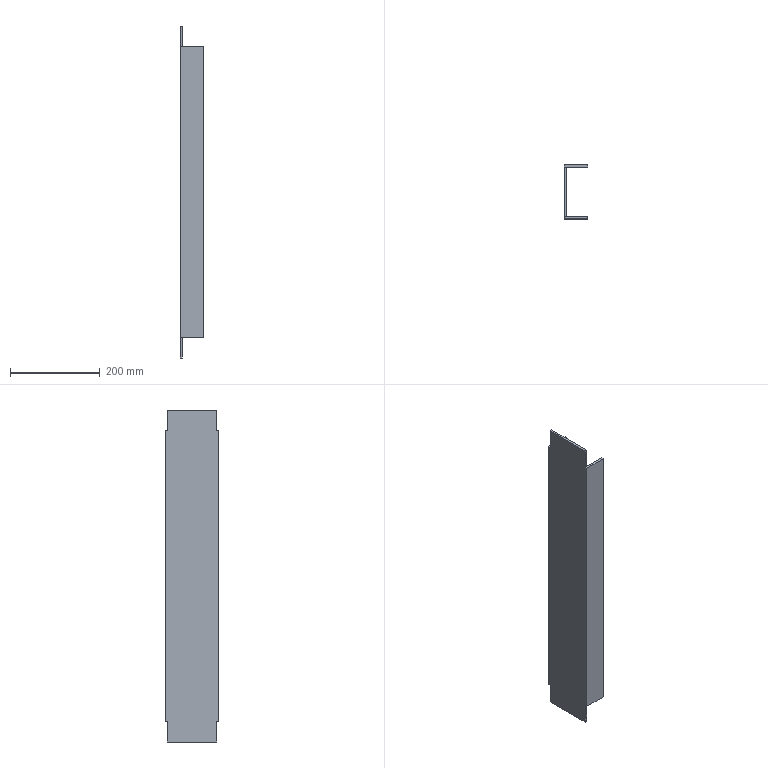Part | SolidWorks | features ICE 3, Extrusion 1 | 1 solid | 18 faces | box 53 x 120 x 740 mm | volume 751500 mm3 | plane 18
STEP:
#1=CARTESIAN_POINT('',(0.,-120.,695.));
#2=VERTEX_POINT('',#1);
#3=CARTESIAN_POINT('',(53.,-120.,695.));
#4=VERTEX_POINT('',#3);
#5=CARTESIAN_POINT('',(53.,-120.,695.));
#6=DIRECTION('',(1.,0.,0.));
#7=VECTOR('',#6,1000.);
#8=LINE('',#5,#7);
#9=EDGE_CURVE('',#2,#4,#8,.T.);
#10=ORIENTED_EDGE('',*,*,#9,.F.);
#11=CARTESIAN_POINT('',(0.,-120.,45.));
#12=VERTEX_POINT('',#11);
#13=CARTESIAN_POINT('',(0.,-120.,740.));
#14=DIRECTION('',(0.,0.,-1.));
#15=VECTOR('',#14,1000.);
#16=LINE('',#13,#15);
#17=EDGE_CURVE('',#2,#12,#16,.T.);
#18=ORIENTED_EDGE('',*,*,#17,.T.);
#19=CARTESIAN_POINT('',(53.,-120.,45.));
#20=VERTEX_POINT('',#19);
#21=CARTESIAN_POINT('',(0.,-120.,45.));
#22=DIRECTION('',(-1.,0.,0.));
#23=VECTOR('',#22,1000.);
#24=LINE('',#21,#23);
#25=EDGE_CURVE('',#20,#12,#24,.T.);
#26=ORIENTED_EDGE('',*,*,#25,.F.);
#27=CARTESIAN_POINT('',(53.,-120.,740.));
#28=DIRECTION('',(0.,0.,-1.));
#29=VECTOR('',#28,1000.);
#30=LINE('',#27,#29);
#31=EDGE_CURVE('',#4,#20,#30,.T.);
#32=ORIENTED_EDGE('',*,*,#31,.F.);
#33=EDGE_LOOP('',(#10,#18,#26,#32));
#34=FACE_OUTER_BOUND('',#33,.T.);
#35=CARTESIAN_POINT('',(0.,-120.,740.));
#36=DIRECTION('',(0.,1.,0.));
#37=DIRECTION('',(0.,0.,1.));
#38=AXIS2_PLACEMENT_3D('',#35,#36,#37);
#39=PLANE('',#38);
#40=ADVANCED_FACE('',(#34),#39,.F.);
#41=CARTESIAN_POINT('',(53.,-115.,695.));
#42=VERTEX_POINT('',#41);
#43=CARTESIAN_POINT('',(53.,-120.,695.));
#44=DIRECTION('',(0.,1.,0.));
#45=VECTOR('',#44,1000.);
#46=LINE('',#43,#45);
#47=EDGE_CURVE('',#4,#42,#46,.T.);
#48=ORIENTED_EDGE('',*,*,#47,.F.);
#49=ORIENTED_EDGE('',*,*,#31,.T.);
#50=CARTESIAN_POINT('',(53.,-115.,45.));
#51=VERTEX_POINT('',#50);
#52=CARTESIAN_POINT('',(53.,-120.,45.));
#53=DIRECTION('',(0.,-1.,0.));
#54=VECTOR('',#53,1000.);
#55=LINE('',#52,#54);
#56=EDGE_CURVE('',#51,#20,#55,.T.);
#57=ORIENTED_EDGE('',*,*,#56,.F.);
#58=CARTESIAN_POINT('',(53.,-115.,740.));
#59=DIRECTION('',(0.,0.,-1.));
#60=VECTOR('',#59,1000.);
#61=LINE('',#58,#60);
#62=EDGE_CURVE('',#42,#51,#61,.T.);
#63=ORIENTED_EDGE('',*,*,#62,.F.);
#64=EDGE_LOOP('',(#48,#49,#57,#63));
#65=FACE_OUTER_BOUND('',#64,.T.);
#66=CARTESIAN_POINT('',(53.,-120.,740.));
#67=DIRECTION('',(-1.,0.,0.));
#68=DIRECTION('',(0.,0.,1.));
#69=AXIS2_PLACEMENT_3D('',#66,#67,#68);
#70=PLANE('',#69);
#71=ADVANCED_FACE('',(#65),#70,.F.);
#72=CARTESIAN_POINT('',(5.,-115.,695.));
#73=VERTEX_POINT('',#72);
#74=CARTESIAN_POINT('',(53.,-115.,695.));
#75=DIRECTION('',(-1.,0.,0.));
#76=VECTOR('',#75,1000.);
#77=LINE('',#74,#76);
#78=EDGE_CURVE('',#42,#73,#77,.T.);
#79=ORIENTED_EDGE('',*,*,#78,.F.);
#80=ORIENTED_EDGE('',*,*,#62,.T.);
#81=CARTESIAN_POINT('',(5.,-115.,45.));
#82=VERTEX_POINT('',#81);
#83=CARTESIAN_POINT('',(53.,-115.,45.));
#84=DIRECTION('',(1.,0.,0.));
#85=VECTOR('',#84,1000.);
#86=LINE('',#83,#85);
#87=EDGE_CURVE('',#82,#51,#86,.T.);
#88=ORIENTED_EDGE('',*,*,#87,.F.);
#89=CARTESIAN_POINT('',(5.,-115.,740.));
#90=DIRECTION('',(0.,0.,-1.));
#91=VECTOR('',#90,1000.);
#92=LINE('',#89,#91);
#93=EDGE_CURVE('',#73,#82,#92,.T.);
#94=ORIENTED_EDGE('',*,*,#93,.F.);
#95=EDGE_LOOP('',(#79,#80,#88,#94));
#96=FACE_OUTER_BOUND('',#95,.T.);
#97=CARTESIAN_POINT('',(5.,-115.,740.));
#98=DIRECTION('',(0.,-1.,0.));
#99=DIRECTION('',(0.,0.,-1.));
#100=AXIS2_PLACEMENT_3D('',#97,#98,#99);
#101=PLANE('',#100);
#102=ADVANCED_FACE('',(#96),#101,.F.);
#103=CARTESIAN_POINT('',(53.,0.,695.));
#104=VERTEX_POINT('',#103);
#105=CARTESIAN_POINT('',(0.,0.,695.));
#106=VERTEX_POINT('',#105);
#107=CARTESIAN_POINT('',(53.,0.,695.));
#108=DIRECTION('',(-1.,0.,0.));
#109=VECTOR('',#108,1000.);
#110=LINE('',#107,#109);
#111=EDGE_CURVE('',#104,#106,#110,.T.);
#112=ORIENTED_EDGE('',*,*,#111,.F.);
#113=CARTESIAN_POINT('',(53.,0.,45.));
#114=VERTEX_POINT('',#113);
#115=CARTESIAN_POINT('',(53.,0.,740.));
#116=DIRECTION('',(0.,0.,-1.));
#117=VECTOR('',#116,1000.);
#118=LINE('',#115,#117);
#119=EDGE_CURVE('',#104,#114,#118,.T.);
#120=ORIENTED_EDGE('',*,*,#119,.T.);
#121=CARTESIAN_POINT('',(0.,0.,45.));
#122=VERTEX_POINT('',#121);
#123=CARTESIAN_POINT('',(53.,0.,45.));
#124=DIRECTION('',(1.,0.,0.));
#125=VECTOR('',#124,1000.);
#126=LINE('',#123,#125);
#127=EDGE_CURVE('',#122,#114,#126,.T.);
#128=ORIENTED_EDGE('',*,*,#127,.F.);
#129=CARTESIAN_POINT('',(0.,0.,740.));
#130=DIRECTION('',(0.,0.,-1.));
#131=VECTOR('',#130,1000.);
#132=LINE('',#129,#131);
#133=EDGE_CURVE('',#106,#122,#132,.T.);
#134=ORIENTED_EDGE('',*,*,#133,.F.);
#135=EDGE_LOOP('',(#112,#120,#128,#134));
#136=FACE_OUTER_BOUND('',#135,.T.);
#137=CARTESIAN_POINT('',(0.,0.,740.));
#138=DIRECTION('',(0.,-1.,0.));
#139=DIRECTION('',(0.,0.,-1.));
#140=AXIS2_PLACEMENT_3D('',#137,#138,#139);
#141=PLANE('',#140);
#142=ADVANCED_FACE('',(#136),#141,.F.);
#143=CARTESIAN_POINT('',(5.,-5.,695.));
#144=VERTEX_POINT('',#143);
#145=CARTESIAN_POINT('',(53.,-5.,695.));
#146=VERTEX_POINT('',#145);
#147=CARTESIAN_POINT('',(0.,-5.,695.));
#148=DIRECTION('',(1.,0.,0.));
#149=VECTOR('',#148,1000.);
#150=LINE('',#147,#149);
#151=EDGE_CURVE('',#144,#146,#150,.T.);
#152=ORIENTED_EDGE('',*,*,#151,.F.);
#153=CARTESIAN_POINT('',(5.,-5.,45.));
#154=VERTEX_POINT('',#153);
#155=CARTESIAN_POINT('',(5.,-5.,740.));
#156=DIRECTION('',(0.,0.,-1.));
#157=VECTOR('',#156,1000.);
#158=LINE('',#155,#157);
#159=EDGE_CURVE('',#144,#154,#158,.T.);
#160=ORIENTED_EDGE('',*,*,#159,.T.);
#161=CARTESIAN_POINT('',(53.,-5.,45.));
#162=VERTEX_POINT('',#161);
#163=CARTESIAN_POINT('',(0.,-5.,45.));
#164=DIRECTION('',(-1.,0.,0.));
#165=VECTOR('',#164,1000.);
#166=LINE('',#163,#165);
#167=EDGE_CURVE('',#162,#154,#166,.T.);
#168=ORIENTED_EDGE('',*,*,#167,.F.);
#169=CARTESIAN_POINT('',(53.,-5.,740.));
#170=DIRECTION('',(0.,0.,-1.));
#171=VECTOR('',#170,1000.);
#172=LINE('',#169,#171);
#173=EDGE_CURVE('',#146,#162,#172,.T.);
#174=ORIENTED_EDGE('',*,*,#173,.F.);
#175=EDGE_LOOP('',(#152,#160,#168,#174));
#176=FACE_OUTER_BOUND('',#175,.T.);
#177=CARTESIAN_POINT('',(5.,-5.,740.));
#178=DIRECTION('',(0.,1.,0.));
#179=DIRECTION('',(0.,0.,1.));
#180=AXIS2_PLACEMENT_3D('',#177,#178,#179);
#181=PLANE('',#180);
#182=ADVANCED_FACE('',(#176),#181,.F.);
#183=CARTESIAN_POINT('',(53.,-5.,695.));
#184=DIRECTION('',(0.,1.,0.));
#185=VECTOR('',#184,1000.);
#186=LINE('',#183,#185);
#187=EDGE_CURVE('',#146,#104,#186,.T.);
#188=ORIENTED_EDGE('',*,*,#187,.F.);
#189=ORIENTED_EDGE('',*,*,#173,.T.);
#190=CARTESIAN_POINT('',(53.,-5.,45.));
#191=DIRECTION('',(0.,-1.,0.));
#192=VECTOR('',#191,1000.);
#193=LINE('',#190,#192);
#194=EDGE_CURVE('',#114,#162,#193,.T.);
#195=ORIENTED_EDGE('',*,*,#194,.F.);
#196=ORIENTED_EDGE('',*,*,#119,.F.);
#197=EDGE_LOOP('',(#188,#189,#195,#196));
#198=FACE_OUTER_BOUND('',#197,.T.);
#199=CARTESIAN_POINT('',(53.,-5.,740.));
#200=DIRECTION('',(-1.,0.,0.));
#201=DIRECTION('',(0.,0.,1.));
#202=AXIS2_PLACEMENT_3D('',#199,#200,#201);
#203=PLANE('',#202);
#204=ADVANCED_FACE('',(#198),#203,.F.);
#205=CARTESIAN_POINT('',(0.,-115.,695.));
#206=VERTEX_POINT('',#205);
#207=CARTESIAN_POINT('',(0.,-115.,695.));
#208=DIRECTION('',(0.,-1.,0.));
#209=VECTOR('',#208,1000.);
#210=LINE('',#207,#209);
#211=EDGE_CURVE('',#206,#2,#210,.T.);
#212=ORIENTED_EDGE('',*,*,#211,.F.);
#213=CARTESIAN_POINT('',(0.,-115.,740.));
#214=VERTEX_POINT('',#213);
#215=CARTESIAN_POINT('',(0.,-115.,695.));
#216=DIRECTION('',(0.,0.,1.));
#217=VECTOR('',#216,1000.);
#218=LINE('',#215,#217);
#219=EDGE_CURVE('',#206,#214,#218,.T.);
#220=ORIENTED_EDGE('',*,*,#219,.T.);
#221=CARTESIAN_POINT('',(0.,-5.,740.));
#222=VERTEX_POINT('',#221);
#223=CARTESIAN_POINT('',(0.,0.,740.));
#224=DIRECTION('',(0.,-1.,0.));
#225=VECTOR('',#224,1000.);
#226=LINE('',#223,#225);
#227=EDGE_CURVE('',#222,#214,#226,.T.);
#228=ORIENTED_EDGE('',*,*,#227,.F.);
#229=CARTESIAN_POINT('',(0.,-5.,695.));
#230=VERTEX_POINT('',#229);
#231=CARTESIAN_POINT('',(0.,-5.,695.));
#232=DIRECTION('',(0.,0.,1.));
#233=VECTOR('',#232,1000.);
#234=LINE('',#231,#233);
#235=EDGE_CURVE('',#230,#222,#234,.T.);
#236=ORIENTED_EDGE('',*,*,#235,.F.);
#237=CARTESIAN_POINT('',(0.,0.,695.));
#238=DIRECTION('',(0.,-1.,0.));
#239=VECTOR('',#238,1000.);
#240=LINE('',#237,#239);
#241=EDGE_CURVE('',#106,#230,#240,.T.);
#242=ORIENTED_EDGE('',*,*,#241,.F.);
#243=ORIENTED_EDGE('',*,*,#133,.T.);
#244=CARTESIAN_POINT('',(0.,-5.,45.));
#245=VERTEX_POINT('',#244);
#246=CARTESIAN_POINT('',(0.,0.,45.));
#247=DIRECTION('',(0.,1.,0.));
#248=VECTOR('',#247,1000.);
#249=LINE('',#246,#248);
#250=EDGE_CURVE('',#245,#122,#249,.T.);
#251=ORIENTED_EDGE('',*,*,#250,.F.);
#252=CARTESIAN_POINT('',(0.,-5.,0.));
#253=VERTEX_POINT('',#252);
#254=CARTESIAN_POINT('',(0.,-5.,45.));
#255=DIRECTION('',(0.,0.,-1.));
#256=VECTOR('',#255,1000.);
#257=LINE('',#254,#256);
#258=EDGE_CURVE('',#245,#253,#257,.T.);
#259=ORIENTED_EDGE('',*,*,#258,.T.);
#260=CARTESIAN_POINT('',(0.,-115.,0.));
#261=VERTEX_POINT('',#260);
#262=CARTESIAN_POINT('',(0.,0.,0.));
#263=DIRECTION('',(0.,-1.,0.));
#264=VECTOR('',#263,1000.);
#265=LINE('',#262,#264);
#266=EDGE_CURVE('',#253,#261,#265,.T.);
#267=ORIENTED_EDGE('',*,*,#266,.T.);
#268=CARTESIAN_POINT('',(0.,-115.,45.));
#269=VERTEX_POINT('',#268);
#270=CARTESIAN_POINT('',(0.,-115.,45.));
#271=DIRECTION('',(0.,0.,-1.));
#272=VECTOR('',#271,1000.);
#273=LINE('',#270,#272);
#274=EDGE_CURVE('',#269,#261,#273,.T.);
#275=ORIENTED_EDGE('',*,*,#274,.F.);
#276=CARTESIAN_POINT('',(0.,-115.,45.));
#277=DIRECTION('',(0.,1.,0.));
#278=VECTOR('',#277,1000.);
#279=LINE('',#276,#278);
#280=EDGE_CURVE('',#12,#269,#279,.T.);
#281=ORIENTED_EDGE('',*,*,#280,.F.);
#282=ORIENTED_EDGE('',*,*,#17,.F.);
#283=EDGE_LOOP('',(#212,#220,#228,#236,#242,#243,#251,#259,#267,#275,#281,#282));
#284=FACE_OUTER_BOUND('',#283,.T.);
#285=CARTESIAN_POINT('',(0.,0.,740.));
#286=DIRECTION('',(1.,0.,0.));
#287=DIRECTION('',(0.,1.,0.));
#288=AXIS2_PLACEMENT_3D('',#285,#286,#287);
#289=PLANE('',#288);
#290=ADVANCED_FACE('',(#284),#289,.F.);
#291=CARTESIAN_POINT('',(5.,-115.,0.));
#292=VERTEX_POINT('',#291);
#293=CARTESIAN_POINT('',(5.,-5.,0.));
#294=VERTEX_POINT('',#293);
#295=CARTESIAN_POINT('',(5.,-5.,0.));
#296=DIRECTION('',(0.,1.,0.));
#297=VECTOR('',#296,1000.);
#298=LINE('',#295,#297);
#299=EDGE_CURVE('',#292,#294,#298,.T.);
#300=ORIENTED_EDGE('',*,*,#299,.T.);
#301=CARTESIAN_POINT('',(5.,-5.,740.));
#302=DIRECTION('',(0.,0.,1.));
#303=VECTOR('',#302,1000.);
#304=LINE('',#301,#303);
#305=EDGE_CURVE('',#294,#154,#304,.T.);
#306=ORIENTED_EDGE('',*,*,#305,.T.);
#307=ORIENTED_EDGE('',*,*,#159,.F.);
#308=CARTESIAN_POINT('',(5.,-5.,740.));
#309=VERTEX_POINT('',#308);
#310=CARTESIAN_POINT('',(5.,-5.,740.));
#311=DIRECTION('',(0.,0.,-1.));
#312=VECTOR('',#311,1000.);
#313=LINE('',#310,#312);
#314=EDGE_CURVE('',#309,#144,#313,.T.);
#315=ORIENTED_EDGE('',*,*,#314,.F.);
#316=CARTESIAN_POINT('',(5.,-115.,740.));
#317=VERTEX_POINT('',#316);
#318=CARTESIAN_POINT('',(5.,-5.,740.));
#319=DIRECTION('',(0.,1.,0.));
#320=VECTOR('',#319,1000.);
#321=LINE('',#318,#320);
#322=EDGE_CURVE('',#317,#309,#321,.T.);
#323=ORIENTED_EDGE('',*,*,#322,.F.);
#324=CARTESIAN_POINT('',(5.,-115.,740.));
#325=DIRECTION('',(0.,0.,-1.));
#326=VECTOR('',#325,1000.);
#327=LINE('',#324,#326);
#328=EDGE_CURVE('',#317,#73,#327,.T.);
#329=ORIENTED_EDGE('',*,*,#328,.T.);
#330=ORIENTED_EDGE('',*,*,#93,.T.);
#331=CARTESIAN_POINT('',(5.,-115.,740.));
#332=DIRECTION('',(0.,0.,-1.));
#333=VECTOR('',#332,1000.);
#334=LINE('',#331,#333);
#335=EDGE_CURVE('',#82,#292,#334,.T.);
#336=ORIENTED_EDGE('',*,*,#335,.T.);
#337=EDGE_LOOP('',(#300,#306,#307,#315,#323,#329,#330,#336));
#338=FACE_OUTER_BOUND('',#337,.T.);
#339=CARTESIAN_POINT('',(5.,-5.,740.));
#340=DIRECTION('',(-1.,0.,0.));
#341=DIRECTION('',(0.,0.,1.));
#342=AXIS2_PLACEMENT_3D('',#339,#340,#341);
#343=PLANE('',#342);
#344=ADVANCED_FACE('',(#338),#343,.F.);
#345=CARTESIAN_POINT('',(0.,-115.,740.));
#346=DIRECTION('',(-1.,0.,0.));
#347=VECTOR('',#346,1000.);
#348=LINE('',#345,#347);
#349=EDGE_CURVE('',#317,#214,#348,.T.);
#350=ORIENTED_EDGE('',*,*,#349,.F.);
#351=ORIENTED_EDGE('',*,*,#322,.T.);
#352=CARTESIAN_POINT('',(0.,-5.,740.));
#353=DIRECTION('',(1.,0.,0.));
#354=VECTOR('',#353,1000.);
#355=LINE('',#352,#354);
#356=EDGE_CURVE('',#222,#309,#355,.T.);
#357=ORIENTED_EDGE('',*,*,#356,.F.);
#358=ORIENTED_EDGE('',*,*,#227,.T.);
#359=EDGE_LOOP('',(#350,#351,#357,#358));
#360=FACE_OUTER_BOUND('',#359,.T.);
#361=CARTESIAN_POINT('',(0.,0.,740.));
#362=DIRECTION('',(0.,0.,1.));
#363=DIRECTION('',(1.,0.,0.));
#364=AXIS2_PLACEMENT_3D('',#361,#362,#363);
#365=PLANE('',#364);
#366=ADVANCED_FACE('',(#360),#365,.T.);
#367=ORIENTED_EDGE('',*,*,#299,.F.);
#368=CARTESIAN_POINT('',(53.,-115.,0.));
#369=DIRECTION('',(1.,0.,0.));
#370=VECTOR('',#369,1000.);
#371=LINE('',#368,#370);
#372=EDGE_CURVE('',#261,#292,#371,.T.);
#373=ORIENTED_EDGE('',*,*,#372,.F.);
#374=ORIENTED_EDGE('',*,*,#266,.F.);
#375=CARTESIAN_POINT('',(0.,-5.,0.));
#376=DIRECTION('',(1.,0.,0.));
#377=VECTOR('',#376,1000.);
#378=LINE('',#375,#377);
#379=EDGE_CURVE('',#253,#294,#378,.T.);
#380=ORIENTED_EDGE('',*,*,#379,.T.);
#381=EDGE_LOOP('',(#367,#373,#374,#380));
#382=FACE_OUTER_BOUND('',#381,.T.);
#383=CARTESIAN_POINT('',(0.,0.,0.));
#384=DIRECTION('',(0.,0.,1.));
#385=DIRECTION('',(1.,0.,0.));
#386=AXIS2_PLACEMENT_3D('',#383,#384,#385);
#387=PLANE('',#386);
#388=ADVANCED_FACE('',(#382),#387,.F.);
#389=ORIENTED_EDGE('',*,*,#379,.F.);
#390=ORIENTED_EDGE('',*,*,#258,.F.);
#391=CARTESIAN_POINT('',(0.,-5.,45.));
#392=DIRECTION('',(-1.,0.,0.));
#393=VECTOR('',#392,1000.);
#394=LINE('',#391,#393);
#395=EDGE_CURVE('',#154,#245,#394,.T.);
#396=ORIENTED_EDGE('',*,*,#395,.F.);
#397=ORIENTED_EDGE('',*,*,#305,.F.);
#398=EDGE_LOOP('',(#389,#390,#396,#397));
#399=FACE_OUTER_BOUND('',#398,.T.);
#400=CARTESIAN_POINT('',(0.,-5.,45.));
#401=DIRECTION('',(0.,-1.,0.));
#402=DIRECTION('',(0.,0.,-1.));
#403=AXIS2_PLACEMENT_3D('',#400,#401,#402);
#404=PLANE('',#403);
#405=ADVANCED_FACE('',(#399),#404,.F.);
#406=ORIENTED_EDGE('',*,*,#194,.T.);
#407=ORIENTED_EDGE('',*,*,#167,.T.);
#408=ORIENTED_EDGE('',*,*,#395,.T.);
#409=ORIENTED_EDGE('',*,*,#250,.T.);
#410=ORIENTED_EDGE('',*,*,#127,.T.);
#411=EDGE_LOOP('',(#406,#407,#408,#409,#410));
#412=FACE_OUTER_BOUND('',#411,.T.);
#413=CARTESIAN_POINT('',(0.,0.,45.));
#414=DIRECTION('',(0.,0.,1.));
#415=DIRECTION('',(1.,0.,0.));
#416=AXIS2_PLACEMENT_3D('',#413,#414,#415);
#417=PLANE('',#416);
#418=ADVANCED_FACE('',(#412),#417,.F.);
#419=CARTESIAN_POINT('',(53.,-115.,45.));
#420=DIRECTION('',(1.,0.,0.));
#421=VECTOR('',#420,1000.);
#422=LINE('',#419,#421);
#423=EDGE_CURVE('',#269,#82,#422,.T.);
#424=ORIENTED_EDGE('',*,*,#423,.F.);
#425=ORIENTED_EDGE('',*,*,#274,.T.);
#426=ORIENTED_EDGE('',*,*,#372,.T.);
#427=ORIENTED_EDGE('',*,*,#335,.F.);
#428=EDGE_LOOP('',(#424,#425,#426,#427));
#429=FACE_OUTER_BOUND('',#428,.T.);
#430=CARTESIAN_POINT('',(53.,-115.,45.));
#431=DIRECTION('',(0.,1.,0.));
#432=DIRECTION('',(0.,0.,1.));
#433=AXIS2_PLACEMENT_3D('',#430,#431,#432);
#434=PLANE('',#433);
#435=ADVANCED_FACE('',(#429),#434,.F.);
#436=ORIENTED_EDGE('',*,*,#56,.T.);
#437=ORIENTED_EDGE('',*,*,#25,.T.);
#438=ORIENTED_EDGE('',*,*,#280,.T.);
#439=ORIENTED_EDGE('',*,*,#423,.T.);
#440=ORIENTED_EDGE('',*,*,#87,.T.);
#441=EDGE_LOOP('',(#436,#437,#438,#439,#440));
#442=FACE_OUTER_BOUND('',#441,.T.);
#443=CARTESIAN_POINT('',(0.,0.,45.));
#444=DIRECTION('',(0.,0.,1.));
#445=DIRECTION('',(1.,0.,0.));
#446=AXIS2_PLACEMENT_3D('',#443,#444,#445);
#447=PLANE('',#446);
#448=ADVANCED_FACE('',(#442),#447,.F.);
#449=CARTESIAN_POINT('',(0.,-5.,695.));
#450=DIRECTION('',(1.,0.,0.));
#451=VECTOR('',#450,1000.);
#452=LINE('',#449,#451);
#453=EDGE_CURVE('',#230,#144,#452,.T.);
#454=ORIENTED_EDGE('',*,*,#453,.F.);
#455=ORIENTED_EDGE('',*,*,#235,.T.);
#456=ORIENTED_EDGE('',*,*,#356,.T.);
#457=ORIENTED_EDGE('',*,*,#314,.T.);
#458=EDGE_LOOP('',(#454,#455,#456,#457));
#459=FACE_OUTER_BOUND('',#458,.T.);
#460=CARTESIAN_POINT('',(0.,-5.,695.));
#461=DIRECTION('',(0.,-1.,0.));
#462=DIRECTION('',(0.,0.,-1.));
#463=AXIS2_PLACEMENT_3D('',#460,#461,#462);
#464=PLANE('',#463);
#465=ADVANCED_FACE('',(#459),#464,.F.);
#466=ORIENTED_EDGE('',*,*,#453,.T.);
#467=ORIENTED_EDGE('',*,*,#151,.T.);
#468=ORIENTED_EDGE('',*,*,#187,.T.);
#469=ORIENTED_EDGE('',*,*,#111,.T.);
#470=ORIENTED_EDGE('',*,*,#241,.T.);
#471=EDGE_LOOP('',(#466,#467,#468,#469,#470));
#472=FACE_OUTER_BOUND('',#471,.T.);
#473=CARTESIAN_POINT('',(0.,0.,695.));
#474=DIRECTION('',(0.,0.,1.));
#475=DIRECTION('',(1.,0.,0.));
#476=AXIS2_PLACEMENT_3D('',#473,#474,#475);
#477=PLANE('',#476);
#478=ADVANCED_FACE('',(#472),#477,.T.);
#479=ORIENTED_EDGE('',*,*,#349,.T.);
#480=ORIENTED_EDGE('',*,*,#219,.F.);
#481=CARTESIAN_POINT('',(53.,-115.,695.));
#482=DIRECTION('',(-1.,0.,0.));
#483=VECTOR('',#482,1000.);
#484=LINE('',#481,#483);
#485=EDGE_CURVE('',#73,#206,#484,.T.);
#486=ORIENTED_EDGE('',*,*,#485,.F.);
#487=ORIENTED_EDGE('',*,*,#328,.F.);
#488=EDGE_LOOP('',(#479,#480,#486,#487));
#489=FACE_OUTER_BOUND('',#488,.T.);
#490=CARTESIAN_POINT('',(53.,-115.,695.));
#491=DIRECTION('',(0.,1.,0.));
#492=DIRECTION('',(0.,0.,1.));
#493=AXIS2_PLACEMENT_3D('',#490,#491,#492);
#494=PLANE('',#493);
#495=ADVANCED_FACE('',(#489),#494,.F.);
#496=ORIENTED_EDGE('',*,*,#47,.T.);
#497=ORIENTED_EDGE('',*,*,#78,.T.);
#498=ORIENTED_EDGE('',*,*,#485,.T.);
#499=ORIENTED_EDGE('',*,*,#211,.T.);
#500=ORIENTED_EDGE('',*,*,#9,.T.);
#501=EDGE_LOOP('',(#496,#497,#498,#499,#500));
#502=FACE_OUTER_BOUND('',#501,.T.);
#503=CARTESIAN_POINT('',(0.,0.,695.));
#504=DIRECTION('',(0.,0.,1.));
#505=DIRECTION('',(1.,0.,0.));
#506=AXIS2_PLACEMENT_3D('',#503,#504,#505);
#507=PLANE('',#506);
#508=ADVANCED_FACE('',(#502),#507,.T.);
#509=CLOSED_SHELL('',(#40,#71,#102,#142,#182,#204,#290,#344,#366,#388,#405,#418,#435,#448,#465,#478,#495,#508));
#510=MANIFOLD_SOLID_BREP('',#509);
#511=CARTESIAN_POINT('',(0.,0.,0.));
#512=DIRECTION('',(0.,0.,1.));
#513=DIRECTION('',(1.,0.,0.));
#514=AXIS2_PLACEMENT_3D('',#511,#512,#513);
#515=(LENGTH_UNIT()NAMED_UNIT(*)SI_UNIT(.MILLI.,.METRE.));
#516=UNCERTAINTY_MEASURE_WITH_UNIT(LENGTH_MEASURE(0.00001),#515,'','');
#517=(NAMED_UNIT(*)PLANE_ANGLE_UNIT()SI_UNIT($,.RADIAN.));
#518=(NAMED_UNIT(*)SI_UNIT($,.STERADIAN.)SOLID_ANGLE_UNIT());
#519=(GEOMETRIC_REPRESENTATION_CONTEXT(3)GLOBAL_UNCERTAINTY_ASSIGNED_CONTEXT((#516))GLOBAL_UNIT_ASSIGNED_CONTEXT((#515,#517,#518))REPRESENTATION_CONTEXT('',''));
#520=ADVANCED_BREP_SHAPE_REPRESENTATION('',(#510,#514),#519);